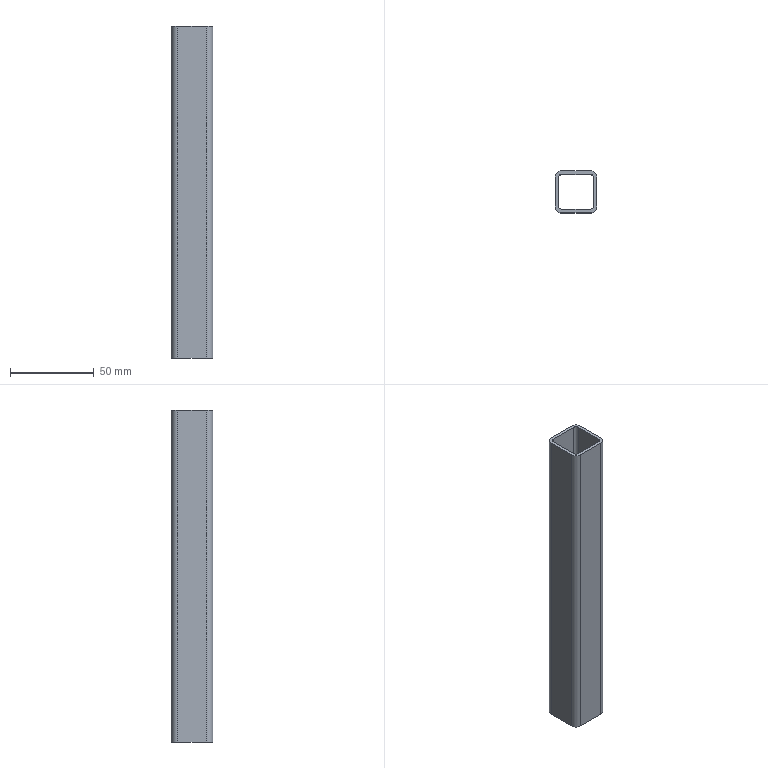Part | SolidWorks | features Extrusion 1 | 1 solid | 18 faces | box 25 x 25 x 198 mm | volume 34392 mm3 | plane 10 | cylinder 8 | commonest cylinder face diameters 4 x4 8 x4
STEP:
#1=CARTESIAN_POINT('',(12.5,8.5,198.));
#2=VERTEX_POINT('',#1);
#3=CARTESIAN_POINT('',(8.5,12.5,198.));
#4=VERTEX_POINT('',#3);
#5=CARTESIAN_POINT('',(8.5,8.5,198.));
#6=DIRECTION('',(0.,0.,1.));
#7=DIRECTION('',(1.,0.,0.));
#8=AXIS2_PLACEMENT_3D('',#5,#6,#7);
#9=CIRCLE('',#8,4.);
#10=EDGE_CURVE('',#2,#4,#9,.T.);
#11=ORIENTED_EDGE('',*,*,#10,.T.);
#12=CARTESIAN_POINT('',(-8.5,12.5,198.));
#13=VERTEX_POINT('',#12);
#14=CARTESIAN_POINT('',(8.5,12.5,198.));
#15=DIRECTION('',(-1.,0.,0.));
#16=VECTOR('',#15,1000.);
#17=LINE('',#14,#16);
#18=EDGE_CURVE('',#4,#13,#17,.T.);
#19=ORIENTED_EDGE('',*,*,#18,.T.);
#20=CARTESIAN_POINT('',(-12.5,8.5,198.));
#21=VERTEX_POINT('',#20);
#22=CARTESIAN_POINT('',(-8.5,8.5,198.));
#23=DIRECTION('',(0.,0.,1.));
#24=DIRECTION('',(1.,0.,0.));
#25=AXIS2_PLACEMENT_3D('',#22,#23,#24);
#26=CIRCLE('',#25,4.);
#27=EDGE_CURVE('',#13,#21,#26,.T.);
#28=ORIENTED_EDGE('',*,*,#27,.T.);
#29=CARTESIAN_POINT('',(-12.5,-8.5,198.));
#30=VERTEX_POINT('',#29);
#31=CARTESIAN_POINT('',(-12.5,-8.5,198.));
#32=DIRECTION('',(0.,-1.,0.));
#33=VECTOR('',#32,1000.);
#34=LINE('',#31,#33);
#35=EDGE_CURVE('',#21,#30,#34,.T.);
#36=ORIENTED_EDGE('',*,*,#35,.T.);
#37=CARTESIAN_POINT('',(-8.5,-12.5,198.));
#38=VERTEX_POINT('',#37);
#39=CARTESIAN_POINT('',(-8.5,-8.5,198.));
#40=DIRECTION('',(0.,0.,1.));
#41=DIRECTION('',(1.,0.,0.));
#42=AXIS2_PLACEMENT_3D('',#39,#40,#41);
#43=CIRCLE('',#42,4.);
#44=EDGE_CURVE('',#30,#38,#43,.T.);
#45=ORIENTED_EDGE('',*,*,#44,.T.);
#46=CARTESIAN_POINT('',(8.5,-12.5,198.));
#47=VERTEX_POINT('',#46);
#48=CARTESIAN_POINT('',(-8.5,-12.5,198.));
#49=DIRECTION('',(1.,0.,0.));
#50=VECTOR('',#49,1000.);
#51=LINE('',#48,#50);
#52=EDGE_CURVE('',#38,#47,#51,.T.);
#53=ORIENTED_EDGE('',*,*,#52,.T.);
#54=CARTESIAN_POINT('',(12.5,-8.5,198.));
#55=VERTEX_POINT('',#54);
#56=CARTESIAN_POINT('',(8.5,-8.5,198.));
#57=DIRECTION('',(0.,0.,1.));
#58=DIRECTION('',(1.,0.,0.));
#59=AXIS2_PLACEMENT_3D('',#56,#57,#58);
#60=CIRCLE('',#59,4.);
#61=EDGE_CURVE('',#47,#55,#60,.T.);
#62=ORIENTED_EDGE('',*,*,#61,.T.);
#63=CARTESIAN_POINT('',(12.5,8.5,198.));
#64=DIRECTION('',(0.,1.,0.));
#65=VECTOR('',#64,1000.);
#66=LINE('',#63,#65);
#67=EDGE_CURVE('',#55,#2,#66,.T.);
#68=ORIENTED_EDGE('',*,*,#67,.T.);
#69=EDGE_LOOP('',(#11,#19,#28,#36,#45,#53,#62,#68));
#70=FACE_OUTER_BOUND('',#69,.T.);
#71=CARTESIAN_POINT('',(-10.5,8.5,198.));
#72=VERTEX_POINT('',#71);
#73=CARTESIAN_POINT('',(-10.5,-8.5,198.));
#74=VERTEX_POINT('',#73);
#75=CARTESIAN_POINT('',(-10.5,-8.5,198.));
#76=DIRECTION('',(0.,-1.,0.));
#77=VECTOR('',#76,1000.);
#78=LINE('',#75,#77);
#79=EDGE_CURVE('',#72,#74,#78,.T.);
#80=ORIENTED_EDGE('',*,*,#79,.F.);
#81=CARTESIAN_POINT('',(-8.5,10.5,198.));
#82=VERTEX_POINT('',#81);
#83=CARTESIAN_POINT('',(-8.5,8.5,198.));
#84=DIRECTION('',(0.,0.,1.));
#85=DIRECTION('',(1.,0.,0.));
#86=AXIS2_PLACEMENT_3D('',#83,#84,#85);
#87=CIRCLE('',#86,2.);
#88=EDGE_CURVE('',#82,#72,#87,.T.);
#89=ORIENTED_EDGE('',*,*,#88,.F.);
#90=CARTESIAN_POINT('',(8.5,10.5,198.));
#91=VERTEX_POINT('',#90);
#92=CARTESIAN_POINT('',(8.5,10.5,198.));
#93=DIRECTION('',(-1.,0.,0.));
#94=VECTOR('',#93,1000.);
#95=LINE('',#92,#94);
#96=EDGE_CURVE('',#91,#82,#95,.T.);
#97=ORIENTED_EDGE('',*,*,#96,.F.);
#98=CARTESIAN_POINT('',(10.5,8.5,198.));
#99=VERTEX_POINT('',#98);
#100=CARTESIAN_POINT('',(8.5,8.5,198.));
#101=DIRECTION('',(0.,0.,1.));
#102=DIRECTION('',(1.,0.,0.));
#103=AXIS2_PLACEMENT_3D('',#100,#101,#102);
#104=CIRCLE('',#103,2.);
#105=EDGE_CURVE('',#99,#91,#104,.T.);
#106=ORIENTED_EDGE('',*,*,#105,.F.);
#107=CARTESIAN_POINT('',(10.5,-8.5,198.));
#108=VERTEX_POINT('',#107);
#109=CARTESIAN_POINT('',(10.5,8.5,198.));
#110=DIRECTION('',(0.,1.,0.));
#111=VECTOR('',#110,1000.);
#112=LINE('',#109,#111);
#113=EDGE_CURVE('',#108,#99,#112,.T.);
#114=ORIENTED_EDGE('',*,*,#113,.F.);
#115=CARTESIAN_POINT('',(8.5,-10.5,198.));
#116=VERTEX_POINT('',#115);
#117=CARTESIAN_POINT('',(8.5,-8.5,198.));
#118=DIRECTION('',(0.,0.,1.));
#119=DIRECTION('',(1.,0.,0.));
#120=AXIS2_PLACEMENT_3D('',#117,#118,#119);
#121=CIRCLE('',#120,2.);
#122=EDGE_CURVE('',#116,#108,#121,.T.);
#123=ORIENTED_EDGE('',*,*,#122,.F.);
#124=CARTESIAN_POINT('',(-8.5,-10.5,198.));
#125=VERTEX_POINT('',#124);
#126=CARTESIAN_POINT('',(-8.5,-10.5,198.));
#127=DIRECTION('',(1.,0.,0.));
#128=VECTOR('',#127,1000.);
#129=LINE('',#126,#128);
#130=EDGE_CURVE('',#125,#116,#129,.T.);
#131=ORIENTED_EDGE('',*,*,#130,.F.);
#132=CARTESIAN_POINT('',(-8.5,-8.5,198.));
#133=DIRECTION('',(0.,0.,1.));
#134=DIRECTION('',(1.,0.,0.));
#135=AXIS2_PLACEMENT_3D('',#132,#133,#134);
#136=CIRCLE('',#135,2.);
#137=EDGE_CURVE('',#74,#125,#136,.T.);
#138=ORIENTED_EDGE('',*,*,#137,.F.);
#139=EDGE_LOOP('',(#80,#89,#97,#106,#114,#123,#131,#138));
#140=FACE_BOUND('',#139,.T.);
#141=CARTESIAN_POINT('',(8.5,8.5,198.));
#142=DIRECTION('',(0.,0.,1.));
#143=DIRECTION('',(1.,0.,0.));
#144=AXIS2_PLACEMENT_3D('',#141,#142,#143);
#145=PLANE('',#144);
#146=ADVANCED_FACE('',(#70,#140),#145,.T.);
#147=CARTESIAN_POINT('',(12.5,8.5,0.));
#148=VERTEX_POINT('',#147);
#149=CARTESIAN_POINT('',(8.5,12.5,0.));
#150=VERTEX_POINT('',#149);
#151=CARTESIAN_POINT('',(8.5,8.5,0.));
#152=DIRECTION('',(0.,0.,1.));
#153=DIRECTION('',(1.,0.,0.));
#154=AXIS2_PLACEMENT_3D('',#151,#152,#153);
#155=CIRCLE('',#154,4.);
#156=EDGE_CURVE('',#148,#150,#155,.T.);
#157=ORIENTED_EDGE('',*,*,#156,.F.);
#158=CARTESIAN_POINT('',(12.5,-8.5,0.));
#159=VERTEX_POINT('',#158);
#160=CARTESIAN_POINT('',(12.5,8.5,0.));
#161=DIRECTION('',(0.,1.,0.));
#162=VECTOR('',#161,1000.);
#163=LINE('',#160,#162);
#164=EDGE_CURVE('',#159,#148,#163,.T.);
#165=ORIENTED_EDGE('',*,*,#164,.F.);
#166=CARTESIAN_POINT('',(8.5,-12.5,0.));
#167=VERTEX_POINT('',#166);
#168=CARTESIAN_POINT('',(8.5,-8.5,0.));
#169=DIRECTION('',(0.,0.,1.));
#170=DIRECTION('',(1.,0.,0.));
#171=AXIS2_PLACEMENT_3D('',#168,#169,#170);
#172=CIRCLE('',#171,4.);
#173=EDGE_CURVE('',#167,#159,#172,.T.);
#174=ORIENTED_EDGE('',*,*,#173,.F.);
#175=CARTESIAN_POINT('',(-8.5,-12.5,0.));
#176=VERTEX_POINT('',#175);
#177=CARTESIAN_POINT('',(-8.5,-12.5,0.));
#178=DIRECTION('',(1.,0.,0.));
#179=VECTOR('',#178,1000.);
#180=LINE('',#177,#179);
#181=EDGE_CURVE('',#176,#167,#180,.T.);
#182=ORIENTED_EDGE('',*,*,#181,.F.);
#183=CARTESIAN_POINT('',(-12.5,-8.5,0.));
#184=VERTEX_POINT('',#183);
#185=CARTESIAN_POINT('',(-8.5,-8.5,0.));
#186=DIRECTION('',(0.,0.,1.));
#187=DIRECTION('',(1.,0.,0.));
#188=AXIS2_PLACEMENT_3D('',#185,#186,#187);
#189=CIRCLE('',#188,4.);
#190=EDGE_CURVE('',#184,#176,#189,.T.);
#191=ORIENTED_EDGE('',*,*,#190,.F.);
#192=CARTESIAN_POINT('',(-12.5,8.5,0.));
#193=VERTEX_POINT('',#192);
#194=CARTESIAN_POINT('',(-12.5,-8.5,0.));
#195=DIRECTION('',(0.,-1.,0.));
#196=VECTOR('',#195,1000.);
#197=LINE('',#194,#196);
#198=EDGE_CURVE('',#193,#184,#197,.T.);
#199=ORIENTED_EDGE('',*,*,#198,.F.);
#200=CARTESIAN_POINT('',(-8.5,12.5,0.));
#201=VERTEX_POINT('',#200);
#202=CARTESIAN_POINT('',(-8.5,8.5,0.));
#203=DIRECTION('',(0.,0.,1.));
#204=DIRECTION('',(1.,0.,0.));
#205=AXIS2_PLACEMENT_3D('',#202,#203,#204);
#206=CIRCLE('',#205,4.);
#207=EDGE_CURVE('',#201,#193,#206,.T.);
#208=ORIENTED_EDGE('',*,*,#207,.F.);
#209=CARTESIAN_POINT('',(8.5,12.5,0.));
#210=DIRECTION('',(-1.,0.,0.));
#211=VECTOR('',#210,1000.);
#212=LINE('',#209,#211);
#213=EDGE_CURVE('',#150,#201,#212,.T.);
#214=ORIENTED_EDGE('',*,*,#213,.F.);
#215=EDGE_LOOP('',(#157,#165,#174,#182,#191,#199,#208,#214));
#216=FACE_OUTER_BOUND('',#215,.T.);
#217=CARTESIAN_POINT('',(-8.5,10.5,0.));
#218=VERTEX_POINT('',#217);
#219=CARTESIAN_POINT('',(-10.5,8.5,0.));
#220=VERTEX_POINT('',#219);
#221=CARTESIAN_POINT('',(-8.5,8.5,0.));
#222=DIRECTION('',(0.,0.,1.));
#223=DIRECTION('',(1.,0.,0.));
#224=AXIS2_PLACEMENT_3D('',#221,#222,#223);
#225=CIRCLE('',#224,2.);
#226=EDGE_CURVE('',#218,#220,#225,.T.);
#227=ORIENTED_EDGE('',*,*,#226,.T.);
#228=CARTESIAN_POINT('',(-10.5,-8.5,0.));
#229=VERTEX_POINT('',#228);
#230=CARTESIAN_POINT('',(-10.5,-8.5,0.));
#231=DIRECTION('',(0.,-1.,0.));
#232=VECTOR('',#231,1000.);
#233=LINE('',#230,#232);
#234=EDGE_CURVE('',#220,#229,#233,.T.);
#235=ORIENTED_EDGE('',*,*,#234,.T.);
#236=CARTESIAN_POINT('',(-8.5,-10.5,0.));
#237=VERTEX_POINT('',#236);
#238=CARTESIAN_POINT('',(-8.5,-8.5,0.));
#239=DIRECTION('',(0.,0.,1.));
#240=DIRECTION('',(1.,0.,0.));
#241=AXIS2_PLACEMENT_3D('',#238,#239,#240);
#242=CIRCLE('',#241,2.);
#243=EDGE_CURVE('',#229,#237,#242,.T.);
#244=ORIENTED_EDGE('',*,*,#243,.T.);
#245=CARTESIAN_POINT('',(8.5,-10.5,0.));
#246=VERTEX_POINT('',#245);
#247=CARTESIAN_POINT('',(-8.5,-10.5,0.));
#248=DIRECTION('',(1.,0.,0.));
#249=VECTOR('',#248,1000.);
#250=LINE('',#247,#249);
#251=EDGE_CURVE('',#237,#246,#250,.T.);
#252=ORIENTED_EDGE('',*,*,#251,.T.);
#253=CARTESIAN_POINT('',(10.5,-8.5,0.));
#254=VERTEX_POINT('',#253);
#255=CARTESIAN_POINT('',(8.5,-8.5,0.));
#256=DIRECTION('',(0.,0.,1.));
#257=DIRECTION('',(1.,0.,0.));
#258=AXIS2_PLACEMENT_3D('',#255,#256,#257);
#259=CIRCLE('',#258,2.);
#260=EDGE_CURVE('',#246,#254,#259,.T.);
#261=ORIENTED_EDGE('',*,*,#260,.T.);
#262=CARTESIAN_POINT('',(10.5,8.5,0.));
#263=VERTEX_POINT('',#262);
#264=CARTESIAN_POINT('',(10.5,8.5,0.));
#265=DIRECTION('',(0.,1.,0.));
#266=VECTOR('',#265,1000.);
#267=LINE('',#264,#266);
#268=EDGE_CURVE('',#254,#263,#267,.T.);
#269=ORIENTED_EDGE('',*,*,#268,.T.);
#270=CARTESIAN_POINT('',(8.5,10.5,0.));
#271=VERTEX_POINT('',#270);
#272=CARTESIAN_POINT('',(8.5,8.5,0.));
#273=DIRECTION('',(0.,0.,1.));
#274=DIRECTION('',(1.,0.,0.));
#275=AXIS2_PLACEMENT_3D('',#272,#273,#274);
#276=CIRCLE('',#275,2.);
#277=EDGE_CURVE('',#263,#271,#276,.T.);
#278=ORIENTED_EDGE('',*,*,#277,.T.);
#279=CARTESIAN_POINT('',(8.5,10.5,0.));
#280=DIRECTION('',(-1.,0.,0.));
#281=VECTOR('',#280,1000.);
#282=LINE('',#279,#281);
#283=EDGE_CURVE('',#271,#218,#282,.T.);
#284=ORIENTED_EDGE('',*,*,#283,.T.);
#285=EDGE_LOOP('',(#227,#235,#244,#252,#261,#269,#278,#284));
#286=FACE_BOUND('',#285,.T.);
#287=CARTESIAN_POINT('',(8.5,8.5,0.));
#288=DIRECTION('',(0.,0.,1.));
#289=DIRECTION('',(1.,0.,0.));
#290=AXIS2_PLACEMENT_3D('',#287,#288,#289);
#291=PLANE('',#290);
#292=ADVANCED_FACE('',(#216,#286),#291,.F.);
#293=ORIENTED_EDGE('',*,*,#156,.T.);
#294=CARTESIAN_POINT('',(8.5,12.5,198.));
#295=DIRECTION('',(0.,0.,-1.));
#296=VECTOR('',#295,1000.);
#297=LINE('',#294,#296);
#298=EDGE_CURVE('',#4,#150,#297,.T.);
#299=ORIENTED_EDGE('',*,*,#298,.F.);
#300=ORIENTED_EDGE('',*,*,#10,.F.);
#301=CARTESIAN_POINT('',(12.5,8.5,198.));
#302=DIRECTION('',(0.,0.,-1.));
#303=VECTOR('',#302,1000.);
#304=LINE('',#301,#303);
#305=EDGE_CURVE('',#2,#148,#304,.T.);
#306=ORIENTED_EDGE('',*,*,#305,.T.);
#307=EDGE_LOOP('',(#293,#299,#300,#306));
#308=FACE_OUTER_BOUND('',#307,.T.);
#309=CARTESIAN_POINT('',(8.5,8.5,198.));
#310=DIRECTION('',(0.,0.,-1.));
#311=DIRECTION('',(-1.,0.,0.));
#312=AXIS2_PLACEMENT_3D('',#309,#310,#311);
#313=CYLINDRICAL_SURFACE('',#312,4.);
#314=ADVANCED_FACE('',(#308),#313,.T.);
#315=ORIENTED_EDGE('',*,*,#213,.T.);
#316=CARTESIAN_POINT('',(-8.5,12.5,198.));
#317=DIRECTION('',(0.,0.,-1.));
#318=VECTOR('',#317,1000.);
#319=LINE('',#316,#318);
#320=EDGE_CURVE('',#13,#201,#319,.T.);
#321=ORIENTED_EDGE('',*,*,#320,.F.);
#322=ORIENTED_EDGE('',*,*,#18,.F.);
#323=ORIENTED_EDGE('',*,*,#298,.T.);
#324=EDGE_LOOP('',(#315,#321,#322,#323));
#325=FACE_OUTER_BOUND('',#324,.T.);
#326=CARTESIAN_POINT('',(8.5,12.5,198.));
#327=DIRECTION('',(0.,-1.,0.));
#328=DIRECTION('',(0.,0.,-1.));
#329=AXIS2_PLACEMENT_3D('',#326,#327,#328);
#330=PLANE('',#329);
#331=ADVANCED_FACE('',(#325),#330,.F.);
#332=ORIENTED_EDGE('',*,*,#207,.T.);
#333=CARTESIAN_POINT('',(-12.5,8.5,198.));
#334=DIRECTION('',(0.,0.,-1.));
#335=VECTOR('',#334,1000.);
#336=LINE('',#333,#335);
#337=EDGE_CURVE('',#21,#193,#336,.T.);
#338=ORIENTED_EDGE('',*,*,#337,.F.);
#339=ORIENTED_EDGE('',*,*,#27,.F.);
#340=ORIENTED_EDGE('',*,*,#320,.T.);
#341=EDGE_LOOP('',(#332,#338,#339,#340));
#342=FACE_OUTER_BOUND('',#341,.T.);
#343=CARTESIAN_POINT('',(-8.5,8.5,198.));
#344=DIRECTION('',(0.,0.,-1.));
#345=DIRECTION('',(-1.,0.,0.));
#346=AXIS2_PLACEMENT_3D('',#343,#344,#345);
#347=CYLINDRICAL_SURFACE('',#346,4.);
#348=ADVANCED_FACE('',(#342),#347,.T.);
#349=ORIENTED_EDGE('',*,*,#198,.T.);
#350=CARTESIAN_POINT('',(-12.5,-8.5,198.));
#351=DIRECTION('',(0.,0.,-1.));
#352=VECTOR('',#351,1000.);
#353=LINE('',#350,#352);
#354=EDGE_CURVE('',#30,#184,#353,.T.);
#355=ORIENTED_EDGE('',*,*,#354,.F.);
#356=ORIENTED_EDGE('',*,*,#35,.F.);
#357=ORIENTED_EDGE('',*,*,#337,.T.);
#358=EDGE_LOOP('',(#349,#355,#356,#357));
#359=FACE_OUTER_BOUND('',#358,.T.);
#360=CARTESIAN_POINT('',(-12.5,-8.5,198.));
#361=DIRECTION('',(1.,0.,0.));
#362=DIRECTION('',(0.,0.,-1.));
#363=AXIS2_PLACEMENT_3D('',#360,#361,#362);
#364=PLANE('',#363);
#365=ADVANCED_FACE('',(#359),#364,.F.);
#366=ORIENTED_EDGE('',*,*,#190,.T.);
#367=CARTESIAN_POINT('',(-8.5,-12.5,198.));
#368=DIRECTION('',(0.,0.,-1.));
#369=VECTOR('',#368,1000.);
#370=LINE('',#367,#369);
#371=EDGE_CURVE('',#38,#176,#370,.T.);
#372=ORIENTED_EDGE('',*,*,#371,.F.);
#373=ORIENTED_EDGE('',*,*,#44,.F.);
#374=ORIENTED_EDGE('',*,*,#354,.T.);
#375=EDGE_LOOP('',(#366,#372,#373,#374));
#376=FACE_OUTER_BOUND('',#375,.T.);
#377=CARTESIAN_POINT('',(-8.5,-8.5,198.));
#378=DIRECTION('',(0.,0.,-1.));
#379=DIRECTION('',(-1.,0.,0.));
#380=AXIS2_PLACEMENT_3D('',#377,#378,#379);
#381=CYLINDRICAL_SURFACE('',#380,4.);
#382=ADVANCED_FACE('',(#376),#381,.T.);
#383=ORIENTED_EDGE('',*,*,#181,.T.);
#384=CARTESIAN_POINT('',(8.5,-12.5,198.));
#385=DIRECTION('',(0.,0.,-1.));
#386=VECTOR('',#385,1000.);
#387=LINE('',#384,#386);
#388=EDGE_CURVE('',#47,#167,#387,.T.);
#389=ORIENTED_EDGE('',*,*,#388,.F.);
#390=ORIENTED_EDGE('',*,*,#52,.F.);
#391=ORIENTED_EDGE('',*,*,#371,.T.);
#392=EDGE_LOOP('',(#383,#389,#390,#391));
#393=FACE_OUTER_BOUND('',#392,.T.);
#394=CARTESIAN_POINT('',(-8.5,-12.5,198.));
#395=DIRECTION('',(0.,1.,0.));
#396=DIRECTION('',(0.,0.,1.));
#397=AXIS2_PLACEMENT_3D('',#394,#395,#396);
#398=PLANE('',#397);
#399=ADVANCED_FACE('',(#393),#398,.F.);
#400=ORIENTED_EDGE('',*,*,#173,.T.);
#401=CARTESIAN_POINT('',(12.5,-8.5,198.));
#402=DIRECTION('',(0.,0.,-1.));
#403=VECTOR('',#402,1000.);
#404=LINE('',#401,#403);
#405=EDGE_CURVE('',#55,#159,#404,.T.);
#406=ORIENTED_EDGE('',*,*,#405,.F.);
#407=ORIENTED_EDGE('',*,*,#61,.F.);
#408=ORIENTED_EDGE('',*,*,#388,.T.);
#409=EDGE_LOOP('',(#400,#406,#407,#408));
#410=FACE_OUTER_BOUND('',#409,.T.);
#411=CARTESIAN_POINT('',(8.5,-8.5,198.));
#412=DIRECTION('',(0.,0.,-1.));
#413=DIRECTION('',(-1.,0.,0.));
#414=AXIS2_PLACEMENT_3D('',#411,#412,#413);
#415=CYLINDRICAL_SURFACE('',#414,4.);
#416=ADVANCED_FACE('',(#410),#415,.T.);
#417=ORIENTED_EDGE('',*,*,#164,.T.);
#418=ORIENTED_EDGE('',*,*,#305,.F.);
#419=ORIENTED_EDGE('',*,*,#67,.F.);
#420=ORIENTED_EDGE('',*,*,#405,.T.);
#421=EDGE_LOOP('',(#417,#418,#419,#420));
#422=FACE_OUTER_BOUND('',#421,.T.);
#423=CARTESIAN_POINT('',(12.5,8.5,198.));
#424=DIRECTION('',(-1.,0.,0.));
#425=DIRECTION('',(0.,0.,1.));
#426=AXIS2_PLACEMENT_3D('',#423,#424,#425);
#427=PLANE('',#426);
#428=ADVANCED_FACE('',(#422),#427,.F.);
#429=ORIENTED_EDGE('',*,*,#226,.F.);
#430=CARTESIAN_POINT('',(-8.5,10.5,198.));
#431=DIRECTION('',(0.,0.,-1.));
#432=VECTOR('',#431,1000.);
#433=LINE('',#430,#432);
#434=EDGE_CURVE('',#82,#218,#433,.T.);
#435=ORIENTED_EDGE('',*,*,#434,.F.);
#436=ORIENTED_EDGE('',*,*,#88,.T.);
#437=CARTESIAN_POINT('',(-10.5,8.5,198.));
#438=DIRECTION('',(0.,0.,-1.));
#439=VECTOR('',#438,1000.);
#440=LINE('',#437,#439);
#441=EDGE_CURVE('',#72,#220,#440,.T.);
#442=ORIENTED_EDGE('',*,*,#441,.T.);
#443=EDGE_LOOP('',(#429,#435,#436,#442));
#444=FACE_OUTER_BOUND('',#443,.T.);
#445=CARTESIAN_POINT('',(-8.5,8.5,198.));
#446=DIRECTION('',(0.,0.,-1.));
#447=DIRECTION('',(-1.,0.,0.));
#448=AXIS2_PLACEMENT_3D('',#445,#446,#447);
#449=CYLINDRICAL_SURFACE('',#448,2.);
#450=ADVANCED_FACE('',(#444),#449,.F.);
#451=ORIENTED_EDGE('',*,*,#234,.F.);
#452=ORIENTED_EDGE('',*,*,#441,.F.);
#453=ORIENTED_EDGE('',*,*,#79,.T.);
#454=CARTESIAN_POINT('',(-10.5,-8.5,198.));
#455=DIRECTION('',(0.,0.,-1.));
#456=VECTOR('',#455,1000.);
#457=LINE('',#454,#456);
#458=EDGE_CURVE('',#74,#229,#457,.T.);
#459=ORIENTED_EDGE('',*,*,#458,.T.);
#460=EDGE_LOOP('',(#451,#452,#453,#459));
#461=FACE_OUTER_BOUND('',#460,.T.);
#462=CARTESIAN_POINT('',(-10.5,-8.5,198.));
#463=DIRECTION('',(1.,0.,0.));
#464=DIRECTION('',(0.,0.,-1.));
#465=AXIS2_PLACEMENT_3D('',#462,#463,#464);
#466=PLANE('',#465);
#467=ADVANCED_FACE('',(#461),#466,.T.);
#468=ORIENTED_EDGE('',*,*,#243,.F.);
#469=ORIENTED_EDGE('',*,*,#458,.F.);
#470=ORIENTED_EDGE('',*,*,#137,.T.);
#471=CARTESIAN_POINT('',(-8.5,-10.5,198.));
#472=DIRECTION('',(0.,0.,-1.));
#473=VECTOR('',#472,1000.);
#474=LINE('',#471,#473);
#475=EDGE_CURVE('',#125,#237,#474,.T.);
#476=ORIENTED_EDGE('',*,*,#475,.T.);
#477=EDGE_LOOP('',(#468,#469,#470,#476));
#478=FACE_OUTER_BOUND('',#477,.T.);
#479=CARTESIAN_POINT('',(-8.5,-8.5,198.));
#480=DIRECTION('',(0.,0.,-1.));
#481=DIRECTION('',(-1.,0.,0.));
#482=AXIS2_PLACEMENT_3D('',#479,#480,#481);
#483=CYLINDRICAL_SURFACE('',#482,2.);
#484=ADVANCED_FACE('',(#478),#483,.F.);
#485=ORIENTED_EDGE('',*,*,#251,.F.);
#486=ORIENTED_EDGE('',*,*,#475,.F.);
#487=ORIENTED_EDGE('',*,*,#130,.T.);
#488=CARTESIAN_POINT('',(8.5,-10.5,198.));
#489=DIRECTION('',(0.,0.,-1.));
#490=VECTOR('',#489,1000.);
#491=LINE('',#488,#490);
#492=EDGE_CURVE('',#116,#246,#491,.T.);
#493=ORIENTED_EDGE('',*,*,#492,.T.);
#494=EDGE_LOOP('',(#485,#486,#487,#493));
#495=FACE_OUTER_BOUND('',#494,.T.);
#496=CARTESIAN_POINT('',(-8.5,-10.5,198.));
#497=DIRECTION('',(0.,1.,0.));
#498=DIRECTION('',(0.,0.,1.));
#499=AXIS2_PLACEMENT_3D('',#496,#497,#498);
#500=PLANE('',#499);
#501=ADVANCED_FACE('',(#495),#500,.T.);
#502=ORIENTED_EDGE('',*,*,#260,.F.);
#503=ORIENTED_EDGE('',*,*,#492,.F.);
#504=ORIENTED_EDGE('',*,*,#122,.T.);
#505=CARTESIAN_POINT('',(10.5,-8.5,198.));
#506=DIRECTION('',(0.,0.,-1.));
#507=VECTOR('',#506,1000.);
#508=LINE('',#505,#507);
#509=EDGE_CURVE('',#108,#254,#508,.T.);
#510=ORIENTED_EDGE('',*,*,#509,.T.);
#511=EDGE_LOOP('',(#502,#503,#504,#510));
#512=FACE_OUTER_BOUND('',#511,.T.);
#513=CARTESIAN_POINT('',(8.5,-8.5,198.));
#514=DIRECTION('',(0.,0.,-1.));
#515=DIRECTION('',(-1.,0.,0.));
#516=AXIS2_PLACEMENT_3D('',#513,#514,#515);
#517=CYLINDRICAL_SURFACE('',#516,2.);
#518=ADVANCED_FACE('',(#512),#517,.F.);
#519=ORIENTED_EDGE('',*,*,#268,.F.);
#520=ORIENTED_EDGE('',*,*,#509,.F.);
#521=ORIENTED_EDGE('',*,*,#113,.T.);
#522=CARTESIAN_POINT('',(10.5,8.5,198.));
#523=DIRECTION('',(0.,0.,-1.));
#524=VECTOR('',#523,1000.);
#525=LINE('',#522,#524);
#526=EDGE_CURVE('',#99,#263,#525,.T.);
#527=ORIENTED_EDGE('',*,*,#526,.T.);
#528=EDGE_LOOP('',(#519,#520,#521,#527));
#529=FACE_OUTER_BOUND('',#528,.T.);
#530=CARTESIAN_POINT('',(10.5,8.5,198.));
#531=DIRECTION('',(-1.,0.,0.));
#532=DIRECTION('',(0.,0.,1.));
#533=AXIS2_PLACEMENT_3D('',#530,#531,#532);
#534=PLANE('',#533);
#535=ADVANCED_FACE('',(#529),#534,.T.);
#536=ORIENTED_EDGE('',*,*,#277,.F.);
#537=ORIENTED_EDGE('',*,*,#526,.F.);
#538=ORIENTED_EDGE('',*,*,#105,.T.);
#539=CARTESIAN_POINT('',(8.5,10.5,198.));
#540=DIRECTION('',(0.,0.,-1.));
#541=VECTOR('',#540,1000.);
#542=LINE('',#539,#541);
#543=EDGE_CURVE('',#91,#271,#542,.T.);
#544=ORIENTED_EDGE('',*,*,#543,.T.);
#545=EDGE_LOOP('',(#536,#537,#538,#544));
#546=FACE_OUTER_BOUND('',#545,.T.);
#547=CARTESIAN_POINT('',(8.5,8.5,198.));
#548=DIRECTION('',(0.,0.,-1.));
#549=DIRECTION('',(-1.,0.,0.));
#550=AXIS2_PLACEMENT_3D('',#547,#548,#549);
#551=CYLINDRICAL_SURFACE('',#550,2.);
#552=ADVANCED_FACE('',(#546),#551,.F.);
#553=ORIENTED_EDGE('',*,*,#283,.F.);
#554=ORIENTED_EDGE('',*,*,#543,.F.);
#555=ORIENTED_EDGE('',*,*,#96,.T.);
#556=ORIENTED_EDGE('',*,*,#434,.T.);
#557=EDGE_LOOP('',(#553,#554,#555,#556));
#558=FACE_OUTER_BOUND('',#557,.T.);
#559=CARTESIAN_POINT('',(8.5,10.5,198.));
#560=DIRECTION('',(0.,-1.,0.));
#561=DIRECTION('',(0.,0.,-1.));
#562=AXIS2_PLACEMENT_3D('',#559,#560,#561);
#563=PLANE('',#562);
#564=ADVANCED_FACE('',(#558),#563,.T.);
#565=CLOSED_SHELL('',(#146,#292,#314,#331,#348,#365,#382,#399,#416,#428,#450,#467,#484,#501,#518,#535,#552,#564));
#566=MANIFOLD_SOLID_BREP('',#565);
#567=CARTESIAN_POINT('',(0.,0.,0.));
#568=DIRECTION('',(0.,0.,1.));
#569=DIRECTION('',(1.,0.,0.));
#570=AXIS2_PLACEMENT_3D('',#567,#568,#569);
#571=(LENGTH_UNIT()NAMED_UNIT(*)SI_UNIT(.MILLI.,.METRE.));
#572=UNCERTAINTY_MEASURE_WITH_UNIT(LENGTH_MEASURE(0.00001),#571,'','');
#573=(NAMED_UNIT(*)PLANE_ANGLE_UNIT()SI_UNIT($,.RADIAN.));
#574=(NAMED_UNIT(*)SI_UNIT($,.STERADIAN.)SOLID_ANGLE_UNIT());
#575=(GEOMETRIC_REPRESENTATION_CONTEXT(3)GLOBAL_UNCERTAINTY_ASSIGNED_CONTEXT((#572))GLOBAL_UNIT_ASSIGNED_CONTEXT((#571,#573,#574))REPRESENTATION_CONTEXT('',''));
#576=ADVANCED_BREP_SHAPE_REPRESENTATION('',(#566,#570),#575);